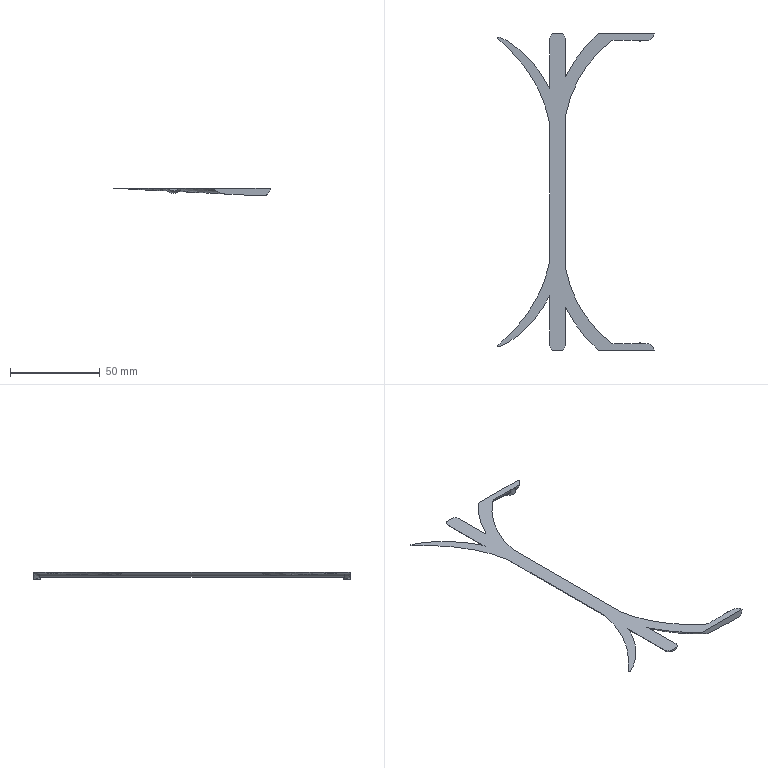Part | STEP file | solid 224 | 1 solid | 32 faces | box 87.441 x 176.873 x 5.302 mm | volume 4897 mm3 | spline 14 | plane 9 | cylinder 5 | sphere 4 | commonest cylinder face diameters 8 x4 10 x1